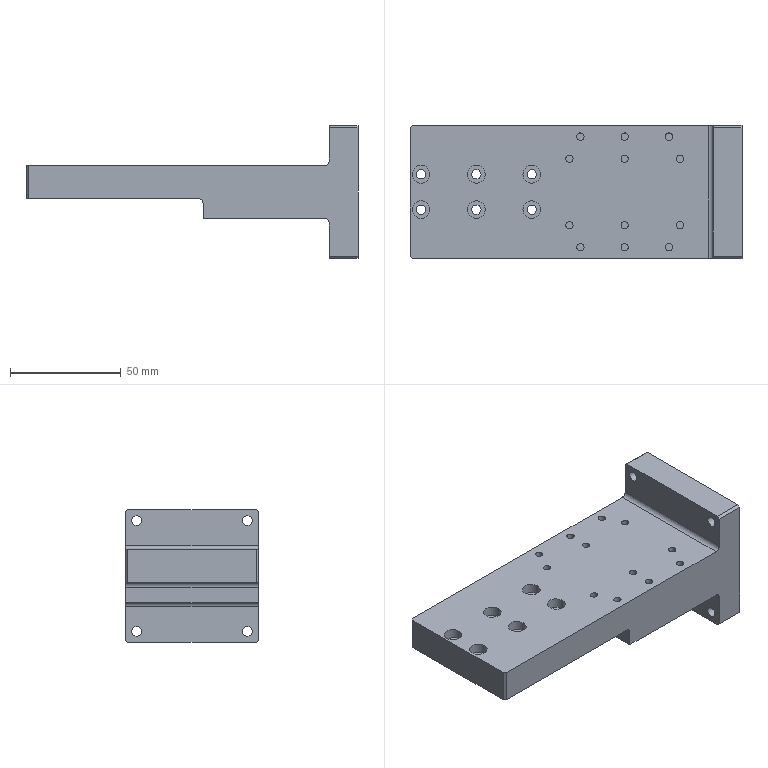NC program | NX | posted with a generic post | part box 150 x 60 x 60 mm
Whole program:
N10 G17 G21 G94 G90
(PLANAR_MILL , TOOL : D10)
N12 T15 M6
N14 G54
N16 G17 G0 G90 X53.4 Y-31.732 B0. C0. S9500 M3
N18 G43 Z30. H15
N20 Z-14.8
N22 G94 G1 Z-15.8 F1000.
N24 X54.9 Y-30.866
N26 G3 X55.4 Y-30. R1.
N28 G1 Y30. F2500.
N30 G3 X54.9 Y30.866 R1.
N32 G1 X53.4 Y31.732
N34 Z-14.8
N36 G0 Z30.
N38 Y-32.021
N40 Z-14.8
N42 G1 Z-15.8 F1000.
N44 X55.4 Y-30.866
N46 G3 X55.9 Y-30. R1.
N48 G1 Y30. F2500.
N50 G3 X55.4 Y30.866 R1.
N52 G1 X53.4 Y32.021
N54 Z-14.8
N56 G0 Z30.
N58 Y-32.309
N60 Z-14.8
N62 G1 Z-15.8 F1000.
N64 X55.9 Y-30.866
N66 G3 X56.4 Y-30. R1.
N68 G1 Y30. F2500.
N70 G3 X55.9 Y30.866 R1.
N72 G1 X53.4 Y32.309
N74 Z-14.8
N76 G0 Z30.
N78 Y-32.598
N80 Z-14.8
N82 G1 Z-15.8 F1000.
N84 X56.4 Y-30.866
N86 G3 X56.9 Y-30. R1.
N88 G1 Y30. F2500.
N90 G3 X56.4 Y30.866 R1.
N92 G1 X53.4 Y32.598
N94 Z-14.8
N96 G0 Z30.
N98 M5
(ZLEVEL_PROFILE_COPY_1_COPY , TOOL : D10JING)
N100 T14 M6
N102 G54
N104 G17 G0 G90 X-76.28 Y35.55 B0. C0. S9500 M3
N106 G43 Z30. H14
N108 Z-17.
N110 G94 G1 Z-20. F1000.
N112 G3 X-74. Y35. R5.
N114 G1 X75. F1200.
N116 G2 X80. Y30. R5.
N118 G1 Y-30.
N120 G2 X75. Y-35. R5.
N122 G1 X-74.
N124 G2 X-77.536 Y-33.536 R5.
N126 G1 X-78.536 Y-32.536
N128 G2 X-80. Y-29. R5.
N130 G1 Y29.
N132 G2 X-78.536 Y32.536 R5.
N134 G1 X-77.536 Y33.536
N136 G2 X-74. Y35. R5.
N138 G3 X-73.134 Y35.5 R1.
N140 G1 X-72.845 Y36.
N142 Z-19.
N144 G0 Z30.
N146 X-76.28 Y35.55
N148 Z-37.
N150 G1 Z-40. F1000.
N152 G3 X-74. Y35. R5.
N154 G1 X75. F1200.
N156 G2 X80. Y30. R5.
N158 G1 Y-30.
N160 G2 X75. Y-35. R5.
N162 G1 X-74.
N164 G2 X-77.536 Y-33.536 R5.
N166 G1 X-78.536 Y-32.536
N168 G2 X-80. Y-29. R5.
N170 G1 Y29.
N172 G2 X-78.536 Y32.536 R5.
N174 G1 X-77.536 Y33.536
N176 G2 X-74. Y35. R5.
N178 G3 X-73.134 Y35.5 R1.
N180 G1 X-72.845 Y36.
N182 Z-39.
N184 G0 Z30.
N186 X-76.28 Y35.55
N188 Z-57.
N190 G1 Z-60. F1000.
N192 G3 X-74. Y35. R5.
N194 G1 X75. F1200.
N196 G2 X80. Y30. R5.
N198 G1 Y-30.
N200 G2 X75. Y-35. R5.
N202 G1 X-74.
N204 G2 X-77.536 Y-33.536 R5.
N206 G1 X-78.536 Y-32.536
N208 G2 X-80. Y-29. R5.
N210 G1 Y29.
N212 G2 X-78.536 Y32.536 R5.
N214 G1 X-77.536 Y33.536
N216 G2 X-74. Y35. R5.
N218 G3 X-73.134 Y35.5 R1.
N220 G1 X-72.845 Y36.
N222 Z-59.
N224 G0 Z30.
(FLOOR_WALL_1_COPY , TOOL : D10JING)
N226 X-74.999 Y-38.
N228 Z-15.
N230 G1 Z-18. F1000.
N232 Y-35.
N234 Y35. F1500.
N236 X-70.018
N238 Y-35.
N240 X-65.038
N242 Y35.
N244 X-60.057
N246 Y-35.
N248 X-55.076
N250 Y35.
N252 X-50.095
N254 Y-35.
N256 X-45.115
N258 Y35.
N260 X-40.134
N262 Y-35.
N264 X-35.153
N266 Y35.
N268 X-30.172
N270 Y-35.
N272 X-25.192
N274 Y35.
N276 X-20.211
N278 Y-35.
N280 X-15.23
N282 Y35.
N284 X-10.25
N286 Y-35.
N288 X-5.269
N290 Y35.
N292 X-0.288
N294 Y-35.
N296 X4.693
N298 Y35.
N300 X9.673
N302 Y-35.
N304 X14.654
N306 Y35.
N308 X19.635
N310 Y-35.
N312 X24.616
N314 Y35.
N316 X29.596
N318 Y-35.
N320 X34.577
N322 Y35.
N324 X39.558
N326 Y-35.
N328 X44.539
N330 Y35.
N332 X49.519
N334 Y-35.
N336 X54.5
N338 Y35.
N340 Y38.
N342 Z-15.
N344 G0 Z30.
N346 X55. Y-38.
N348 Z-15.
N350 G1 Z-18. F1000.
N352 Y-35.
N354 Y35. F1500.
N356 Y38.
N358 Z-15.
N360 G0 Z30.
(HOLE_MILLING , TOOL : D6)
N362 T12 M6
N364 G17 G43 G0 G90 X-70. Y8. Z30. B0. C0. S9500 H12 M3
N366 Z-17.5
N368 G94 G3 X-69.5 Y7.5 R0.5 F1650.
N370 X-69. Y8. R0.5
N372 X-69. Y8. Z-18.1 I-1. J0.
N374 X-69. Y8. Z-18.7 I-1. J0.
N376 X-69. Y8. Z-19.3 I-1. J0.
N378 X-69. Y8. Z-19.9 I-1. J0.
N380 X-69. Y8. Z-20.5 I-1. J0.
N382 X-69. Y8. Z-21.1 I-1. J0.
N384 X-69. Y8. Z-21.7 I-1. J0.
N386 X-69. Y8. Z-22.3 I-1. J0.
N388 X-70.5 Y8.866 Z-22.5 R1.
N390 X-70.866 Y7.5 R1.
N392 X-70.5 Y8.866 R-1.
N394 X-70.683 Y8.183 R0.5
N396 X-70. Y8. R0.5
N398 G0 Z30.
N400 Y-8.
N402 Z-17.5
N404 G3 X-69.5 Y-8.5 R0.5
N406 X-69. Y-8. R0.5
N408 X-69. Y-8. Z-18.1 I-1. J0.
N410 X-69. Y-8. Z-18.7 I-1. J0.
N412 X-69. Y-8. Z-19.3 I-1. J0.
N414 X-69. Y-8. Z-19.9 I-1. J0.
N416 X-69. Y-8. Z-20.5 I-1. J0.
N418 X-69. Y-8. Z-21.1 I-1. J0.
N420 X-69. Y-8. Z-21.7 I-1. J0.
N422 X-69. Y-8. Z-22.3 I-1. J0.
N424 X-70.5 Y-7.134 Z-22.5 R1.
N426 X-70.866 Y-8.5 R1.
N428 X-70.5 Y-7.134 R-1.
N430 X-70.683 Y-7.817 R0.5
N432 X-70. Y-8. R0.5
N434 G0 Z30.
N436 X-45. Y8.
N438 Z-17.5
N440 G3 X-44.5 Y7.5 R0.5
N442 X-44. Y8. R0.5
N444 X-44. Y8. Z-18.1 I-1. J0.
N446 X-44. Y8. Z-18.7 I-1. J0.
N448 X-44. Y8. Z-19.3 I-1. J0.
N450 X-44. Y8. Z-19.9 I-1. J0.
N452 X-44. Y8. Z-20.5 I-1. J0.
N454 X-44. Y8. Z-21.1 I-1. J0.
N456 X-44. Y8. Z-21.7 I-1. J0.
N458 X-44. Y8. Z-22.3 I-1. J0.
N460 X-45.5 Y8.866 Z-22.5 R1.
N462 X-45.866 Y7.5 R1.
N464 X-45.5 Y8.866 R-1.
N466 X-45.683 Y8.183 R0.5
N468 X-45. Y8. R0.5
N470 G0 Z30.
N472 Y-8.
N474 Z-17.5
N476 G3 X-44.5 Y-8.5 R0.5
N478 X-44. Y-8. R0.5
N480 X-44. Y-8. Z-18.1 I-1. J0.
N482 X-44. Y-8. Z-18.7 I-1. J0.
N484 X-44. Y-8. Z-19.3 I-1. J0.
N486 X-44. Y-8. Z-19.9 I-1. J0.
N488 X-44. Y-8. Z-20.5 I-1. J0.
N490 X-44. Y-8. Z-21.1 I-1. J0.
N492 X-44. Y-8. Z-21.7 I-1. J0.
N494 X-44. Y-8. Z-22.3 I-1. J0.
N496 X-45.5 Y-7.134 Z-22.5 R1.
N498 X-45.866 Y-8.5 R1.
N500 X-45.5 Y-7.134 R-1.
N502 X-45.683 Y-7.817 R0.5
N504 X-45. Y-8. R0.5
N506 G0 Z30.
N508 X-20. Y8.
N510 Z-17.5
N512 G3 X-19.5 Y7.5 R0.5
N514 X-19. Y8. R0.5
N516 X-19. Y8. Z-18.1 I-1. J0.
N518 X-19. Y8. Z-18.7 I-1. J0.
N520 X-19. Y8. Z-19.3 I-1. J0.
N522 X-19. Y8. Z-19.9 I-1. J0.
N524 X-19. Y8. Z-20.5 I-1. J0.
N526 X-19. Y8. Z-21.1 I-1. J0.
N528 X-19. Y8. Z-21.7 I-1. J0.
N530 X-19. Y8. Z-22.3 I-1. J0.
N532 X-20.5 Y8.866 Z-22.5 R1.
N534 X-20.866 Y7.5 R1.
N536 X-20.5 Y8.866 R-1.
N538 X-20.683 Y8.183 R0.5
N540 X-20. Y8. R0.5
N542 G0 Z30.
N544 Y-8.
N546 Z-17.5
N548 G3 X-19.5 Y-8.5 R0.5
N550 X-19. Y-8. R0.5
N552 X-19. Y-8. Z-18.1 I-1. J0.
N554 X-19. Y-8. Z-18.7 I-1. J0.
N556 X-19. Y-8. Z-19.3 I-1. J0.
N558 X-19. Y-8. Z-19.9 I-1. J0.
N560 X-19. Y-8. Z-20.5 I-1. J0.
N562 X-19. Y-8. Z-21.1 I-1. J0.
N564 X-19. Y-8. Z-21.7 I-1. J0.
N566 X-19. Y-8. Z-22.3 I-1. J0.
N568 X-20.5 Y-7.134 Z-22.5 R1.
N570 X-20.866 Y-8.5 R1.
N572 X-20.5 Y-7.134 R-1.
N574 X-20.683 Y-7.817 R0.5
N576 X-20. Y-8. R0.5
N578 G0 Z30.
N580 M5
N582 M2